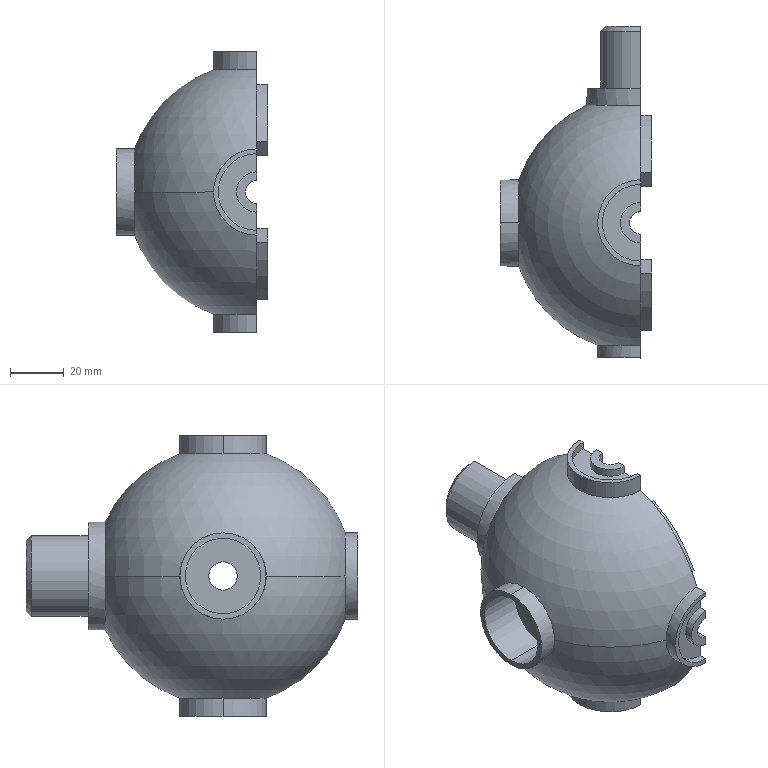Part | SolidWorks | features ICE 15, MirrorPattern 1, RevCut 1, Revolution 1, StudWizard 1 | 1 solid | 69 faces | box 56 x 123 x 104 mm | volume 175814 mm3 | cylinder 34 | plane 30 | sphere 4 | cone 1 | commonest cylinder face diameters 32 x7 8.5 x4 15 x4 28.5 x4 64 x4 88 x4